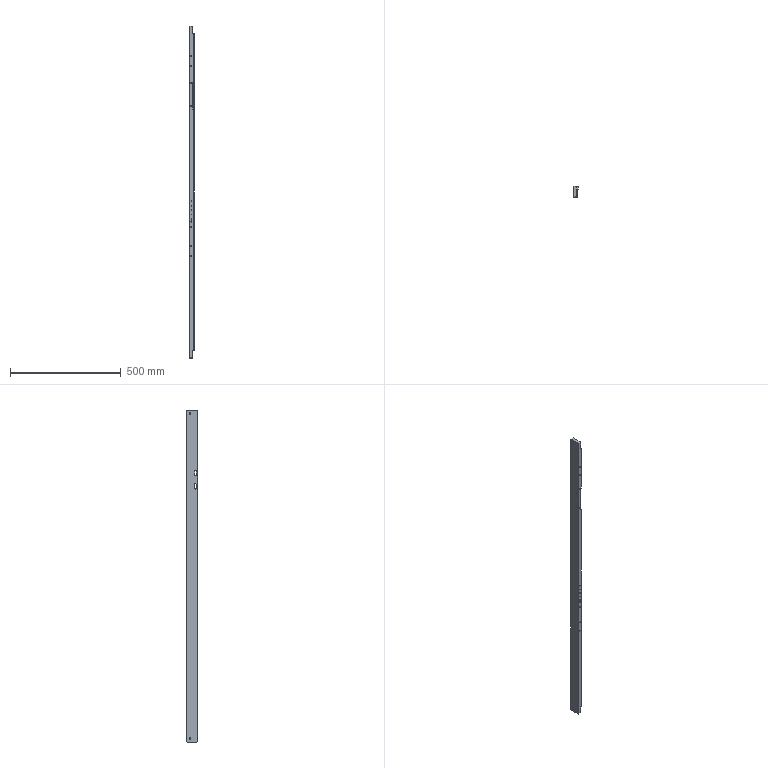Part | SolidWorks | features HoleWzd 7, ICE 4, Chamfer 2, Extrusion 1, Fillet 1 | 1 solid | 109 faces | box 20 x 50 x 1500 mm | volume 1170334 mm3 | cylinder 46 | cone 34 | plane 29 | commonest cylinder face diameters 3.3 x18 5 x16 5.5 x6 6.8 x4 20 x2